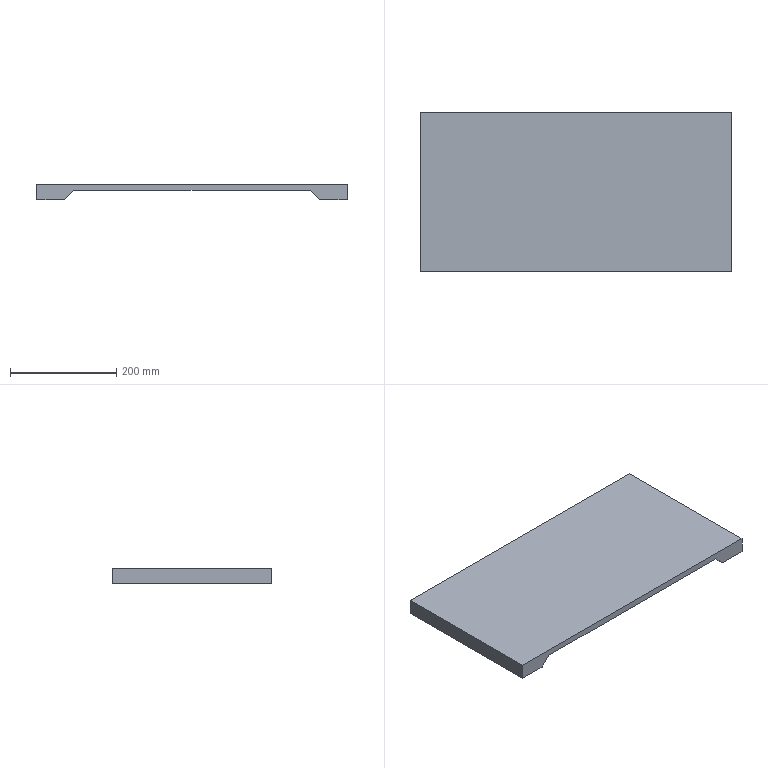Part | STEP file | Platform 2 base plate | 1 solid | 10 faces | box 585 x 300 x 30 mm | volume 2764800 mm3 | plane 10
STEP:
#1=CARTESIAN_POINT('',(240.5,-150.,0.));
#2=VERTEX_POINT('',#1);
#3=CARTESIAN_POINT('',(292.5,-150.,0.));
#4=VERTEX_POINT('',#3);
#5=CARTESIAN_POINT('',(-292.5,-150.,0.));
#6=DIRECTION('',(1.,0.,0.));
#7=VECTOR('',#6,1000.);
#8=LINE('',#5,#7);
#9=EDGE_CURVE('',#2,#4,#8,.T.);
#10=ORIENTED_EDGE('',*,*,#9,.F.);
#11=CARTESIAN_POINT('',(240.5,150.,0.));
#12=VERTEX_POINT('',#11);
#13=CARTESIAN_POINT('',(240.5,150.,0.));
#14=DIRECTION('',(0.,-1.,0.));
#15=VECTOR('',#14,1000.);
#16=LINE('',#13,#15);
#17=EDGE_CURVE('',#12,#2,#16,.T.);
#18=ORIENTED_EDGE('',*,*,#17,.F.);
#19=CARTESIAN_POINT('',(292.5,150.,0.));
#20=VERTEX_POINT('',#19);
#21=CARTESIAN_POINT('',(-292.5,150.,0.));
#22=DIRECTION('',(-1.,0.,0.));
#23=VECTOR('',#22,1000.);
#24=LINE('',#21,#23);
#25=EDGE_CURVE('',#20,#12,#24,.T.);
#26=ORIENTED_EDGE('',*,*,#25,.F.);
#27=CARTESIAN_POINT('',(292.5,150.,0.));
#28=DIRECTION('',(0.,1.,0.));
#29=VECTOR('',#28,1000.);
#30=LINE('',#27,#29);
#31=EDGE_CURVE('',#4,#20,#30,.T.);
#32=ORIENTED_EDGE('',*,*,#31,.F.);
#33=EDGE_LOOP('',(#10,#18,#26,#32));
#34=FACE_OUTER_BOUND('',#33,.T.);
#35=CARTESIAN_POINT('',(0.,0.,0.));
#36=DIRECTION('',(0.,0.,1.));
#37=DIRECTION('',(1.,0.,0.));
#38=AXIS2_PLACEMENT_3D('',#35,#36,#37);
#39=PLANE('',#38);
#40=ADVANCED_FACE('',(#34),#39,.F.);
#41=ORIENTED_EDGE('',*,*,#31,.T.);
#42=CARTESIAN_POINT('',(292.5,150.,30.));
#43=VERTEX_POINT('',#42);
#44=CARTESIAN_POINT('',(292.5,150.,30.));
#45=DIRECTION('',(0.,0.,-1.));
#46=VECTOR('',#45,1000.);
#47=LINE('',#44,#46);
#48=EDGE_CURVE('',#43,#20,#47,.T.);
#49=ORIENTED_EDGE('',*,*,#48,.F.);
#50=CARTESIAN_POINT('',(292.5,-150.,30.));
#51=VERTEX_POINT('',#50);
#52=CARTESIAN_POINT('',(292.5,150.,30.));
#53=DIRECTION('',(0.,1.,0.));
#54=VECTOR('',#53,1000.);
#55=LINE('',#52,#54);
#56=EDGE_CURVE('',#51,#43,#55,.T.);
#57=ORIENTED_EDGE('',*,*,#56,.F.);
#58=CARTESIAN_POINT('',(292.5,-150.,30.));
#59=DIRECTION('',(0.,0.,-1.));
#60=VECTOR('',#59,1000.);
#61=LINE('',#58,#60);
#62=EDGE_CURVE('',#51,#4,#61,.T.);
#63=ORIENTED_EDGE('',*,*,#62,.T.);
#64=EDGE_LOOP('',(#41,#49,#57,#63));
#65=FACE_OUTER_BOUND('',#64,.T.);
#66=CARTESIAN_POINT('',(292.5,150.,30.));
#67=DIRECTION('',(-1.,0.,0.));
#68=DIRECTION('',(0.,0.,1.));
#69=AXIS2_PLACEMENT_3D('',#66,#67,#68);
#70=PLANE('',#69);
#71=ADVANCED_FACE('',(#65),#70,.F.);
#72=ORIENTED_EDGE('',*,*,#25,.T.);
#73=CARTESIAN_POINT('',(222.5,150.,18.));
#74=VERTEX_POINT('',#73);
#75=CARTESIAN_POINT('',(222.5,150.,18.));
#76=DIRECTION('',(-0.7071,0.,0.7071));
#77=VECTOR('',#76,1000.);
#78=LINE('',#75,#77);
#79=EDGE_CURVE('',#12,#74,#78,.T.);
#80=ORIENTED_EDGE('',*,*,#79,.T.);
#81=CARTESIAN_POINT('',(-222.5,150.,18.));
#82=VERTEX_POINT('',#81);
#83=CARTESIAN_POINT('',(-222.5,150.,18.));
#84=DIRECTION('',(-1.,0.,0.));
#85=VECTOR('',#84,1000.);
#86=LINE('',#83,#85);
#87=EDGE_CURVE('',#74,#82,#86,.T.);
#88=ORIENTED_EDGE('',*,*,#87,.T.);
#89=CARTESIAN_POINT('',(-240.5,150.,0.));
#90=VERTEX_POINT('',#89);
#91=CARTESIAN_POINT('',(-222.5,150.,18.));
#92=DIRECTION('',(-0.7071,0.,-0.7071));
#93=VECTOR('',#92,1000.);
#94=LINE('',#91,#93);
#95=EDGE_CURVE('',#82,#90,#94,.T.);
#96=ORIENTED_EDGE('',*,*,#95,.T.);
#97=CARTESIAN_POINT('',(-292.5,150.,0.));
#98=VERTEX_POINT('',#97);
#99=CARTESIAN_POINT('',(-292.5,150.,0.));
#100=DIRECTION('',(-1.,0.,0.));
#101=VECTOR('',#100,1000.);
#102=LINE('',#99,#101);
#103=EDGE_CURVE('',#90,#98,#102,.T.);
#104=ORIENTED_EDGE('',*,*,#103,.T.);
#105=CARTESIAN_POINT('',(-292.5,150.,30.));
#106=VERTEX_POINT('',#105);
#107=CARTESIAN_POINT('',(-292.5,150.,30.));
#108=DIRECTION('',(0.,0.,-1.));
#109=VECTOR('',#108,1000.);
#110=LINE('',#107,#109);
#111=EDGE_CURVE('',#106,#98,#110,.T.);
#112=ORIENTED_EDGE('',*,*,#111,.F.);
#113=CARTESIAN_POINT('',(-292.5,150.,30.));
#114=DIRECTION('',(-1.,0.,0.));
#115=VECTOR('',#114,1000.);
#116=LINE('',#113,#115);
#117=EDGE_CURVE('',#43,#106,#116,.T.);
#118=ORIENTED_EDGE('',*,*,#117,.F.);
#119=ORIENTED_EDGE('',*,*,#48,.T.);
#120=EDGE_LOOP('',(#72,#80,#88,#96,#104,#112,#118,#119));
#121=FACE_OUTER_BOUND('',#120,.T.);
#122=CARTESIAN_POINT('',(-292.5,150.,30.));
#123=DIRECTION('',(0.,-1.,0.));
#124=DIRECTION('',(0.,0.,-1.));
#125=AXIS2_PLACEMENT_3D('',#122,#123,#124);
#126=PLANE('',#125);
#127=ADVANCED_FACE('',(#121),#126,.F.);
#128=CARTESIAN_POINT('',(-292.5,-150.,0.));
#129=VERTEX_POINT('',#128);
#130=CARTESIAN_POINT('',(-292.5,150.,0.));
#131=DIRECTION('',(0.,-1.,0.));
#132=VECTOR('',#131,1000.);
#133=LINE('',#130,#132);
#134=EDGE_CURVE('',#98,#129,#133,.T.);
#135=ORIENTED_EDGE('',*,*,#134,.T.);
#136=CARTESIAN_POINT('',(-292.5,-150.,30.));
#137=VERTEX_POINT('',#136);
#138=CARTESIAN_POINT('',(-292.5,-150.,30.));
#139=DIRECTION('',(0.,0.,-1.));
#140=VECTOR('',#139,1000.);
#141=LINE('',#138,#140);
#142=EDGE_CURVE('',#137,#129,#141,.T.);
#143=ORIENTED_EDGE('',*,*,#142,.F.);
#144=CARTESIAN_POINT('',(-292.5,150.,30.));
#145=DIRECTION('',(0.,-1.,0.));
#146=VECTOR('',#145,1000.);
#147=LINE('',#144,#146);
#148=EDGE_CURVE('',#106,#137,#147,.T.);
#149=ORIENTED_EDGE('',*,*,#148,.F.);
#150=ORIENTED_EDGE('',*,*,#111,.T.);
#151=EDGE_LOOP('',(#135,#143,#149,#150));
#152=FACE_OUTER_BOUND('',#151,.T.);
#153=CARTESIAN_POINT('',(-292.5,150.,30.));
#154=DIRECTION('',(1.,0.,0.));
#155=DIRECTION('',(0.,1.,0.));
#156=AXIS2_PLACEMENT_3D('',#153,#154,#155);
#157=PLANE('',#156);
#158=ADVANCED_FACE('',(#152),#157,.F.);
#159=CARTESIAN_POINT('',(222.5,-150.,18.));
#160=VERTEX_POINT('',#159);
#161=CARTESIAN_POINT('',(-222.5,-150.,18.));
#162=VERTEX_POINT('',#161);
#163=CARTESIAN_POINT('',(-222.5,-150.,18.));
#164=DIRECTION('',(-1.,0.,0.));
#165=VECTOR('',#164,1000.);
#166=LINE('',#163,#165);
#167=EDGE_CURVE('',#160,#162,#166,.T.);
#168=ORIENTED_EDGE('',*,*,#167,.F.);
#169=CARTESIAN_POINT('',(222.5,-150.,18.));
#170=DIRECTION('',(-0.7071,0.,0.7071));
#171=VECTOR('',#170,1000.);
#172=LINE('',#169,#171);
#173=EDGE_CURVE('',#2,#160,#172,.T.);
#174=ORIENTED_EDGE('',*,*,#173,.F.);
#175=ORIENTED_EDGE('',*,*,#9,.T.);
#176=ORIENTED_EDGE('',*,*,#62,.F.);
#177=CARTESIAN_POINT('',(-292.5,-150.,30.));
#178=DIRECTION('',(1.,0.,0.));
#179=VECTOR('',#178,1000.);
#180=LINE('',#177,#179);
#181=EDGE_CURVE('',#137,#51,#180,.T.);
#182=ORIENTED_EDGE('',*,*,#181,.F.);
#183=ORIENTED_EDGE('',*,*,#142,.T.);
#184=CARTESIAN_POINT('',(-240.5,-150.,0.));
#185=VERTEX_POINT('',#184);
#186=CARTESIAN_POINT('',(-292.5,-150.,0.));
#187=DIRECTION('',(1.,0.,0.));
#188=VECTOR('',#187,1000.);
#189=LINE('',#186,#188);
#190=EDGE_CURVE('',#129,#185,#189,.T.);
#191=ORIENTED_EDGE('',*,*,#190,.T.);
#192=CARTESIAN_POINT('',(-222.5,-150.,18.));
#193=DIRECTION('',(-0.7071,0.,-0.7071));
#194=VECTOR('',#193,1000.);
#195=LINE('',#192,#194);
#196=EDGE_CURVE('',#162,#185,#195,.T.);
#197=ORIENTED_EDGE('',*,*,#196,.F.);
#198=EDGE_LOOP('',(#168,#174,#175,#176,#182,#183,#191,#197));
#199=FACE_OUTER_BOUND('',#198,.T.);
#200=CARTESIAN_POINT('',(-292.5,-150.,30.));
#201=DIRECTION('',(0.,1.,0.));
#202=DIRECTION('',(0.,0.,1.));
#203=AXIS2_PLACEMENT_3D('',#200,#201,#202);
#204=PLANE('',#203);
#205=ADVANCED_FACE('',(#199),#204,.F.);
#206=ORIENTED_EDGE('',*,*,#56,.T.);
#207=ORIENTED_EDGE('',*,*,#117,.T.);
#208=ORIENTED_EDGE('',*,*,#148,.T.);
#209=ORIENTED_EDGE('',*,*,#181,.T.);
#210=EDGE_LOOP('',(#206,#207,#208,#209));
#211=FACE_OUTER_BOUND('',#210,.T.);
#212=CARTESIAN_POINT('',(0.,0.,30.));
#213=DIRECTION('',(0.,0.,1.));
#214=DIRECTION('',(1.,0.,0.));
#215=AXIS2_PLACEMENT_3D('',#212,#213,#214);
#216=PLANE('',#215);
#217=ADVANCED_FACE('',(#211),#216,.T.);
#218=ORIENTED_EDGE('',*,*,#103,.F.);
#219=CARTESIAN_POINT('',(-240.5,150.,0.));
#220=DIRECTION('',(0.,-1.,0.));
#221=VECTOR('',#220,1000.);
#222=LINE('',#219,#221);
#223=EDGE_CURVE('',#90,#185,#222,.T.);
#224=ORIENTED_EDGE('',*,*,#223,.T.);
#225=ORIENTED_EDGE('',*,*,#190,.F.);
#226=ORIENTED_EDGE('',*,*,#134,.F.);
#227=EDGE_LOOP('',(#218,#224,#225,#226));
#228=FACE_OUTER_BOUND('',#227,.T.);
#229=CARTESIAN_POINT('',(0.,0.,0.));
#230=DIRECTION('',(0.,0.,1.));
#231=DIRECTION('',(1.,0.,0.));
#232=AXIS2_PLACEMENT_3D('',#229,#230,#231);
#233=PLANE('',#232);
#234=ADVANCED_FACE('',(#228),#233,.F.);
#235=ORIENTED_EDGE('',*,*,#173,.T.);
#236=CARTESIAN_POINT('',(222.5,150.,18.));
#237=DIRECTION('',(0.,-1.,0.));
#238=VECTOR('',#237,1000.);
#239=LINE('',#236,#238);
#240=EDGE_CURVE('',#74,#160,#239,.T.);
#241=ORIENTED_EDGE('',*,*,#240,.F.);
#242=ORIENTED_EDGE('',*,*,#79,.F.);
#243=ORIENTED_EDGE('',*,*,#17,.T.);
#244=EDGE_LOOP('',(#235,#241,#242,#243));
#245=FACE_OUTER_BOUND('',#244,.T.);
#246=CARTESIAN_POINT('',(222.5,150.,18.));
#247=DIRECTION('',(0.7071,0.,0.7071));
#248=DIRECTION('',(0.7071,0.,-0.7071));
#249=AXIS2_PLACEMENT_3D('',#246,#247,#248);
#250=PLANE('',#249);
#251=ADVANCED_FACE('',(#245),#250,.F.);
#252=ORIENTED_EDGE('',*,*,#196,.T.);
#253=ORIENTED_EDGE('',*,*,#223,.F.);
#254=ORIENTED_EDGE('',*,*,#95,.F.);
#255=CARTESIAN_POINT('',(-222.5,150.,18.));
#256=DIRECTION('',(0.,-1.,0.));
#257=VECTOR('',#256,1000.);
#258=LINE('',#255,#257);
#259=EDGE_CURVE('',#82,#162,#258,.T.);
#260=ORIENTED_EDGE('',*,*,#259,.T.);
#261=EDGE_LOOP('',(#252,#253,#254,#260));
#262=FACE_OUTER_BOUND('',#261,.T.);
#263=CARTESIAN_POINT('',(-222.5,150.,18.));
#264=DIRECTION('',(-0.7071,0.,0.7071));
#265=DIRECTION('',(0.7071,0.,0.7071));
#266=AXIS2_PLACEMENT_3D('',#263,#264,#265);
#267=PLANE('',#266);
#268=ADVANCED_FACE('',(#262),#267,.F.);
#269=ORIENTED_EDGE('',*,*,#167,.T.);
#270=ORIENTED_EDGE('',*,*,#259,.F.);
#271=ORIENTED_EDGE('',*,*,#87,.F.);
#272=ORIENTED_EDGE('',*,*,#240,.T.);
#273=EDGE_LOOP('',(#269,#270,#271,#272));
#274=FACE_OUTER_BOUND('',#273,.T.);
#275=CARTESIAN_POINT('',(-222.5,150.,18.));
#276=DIRECTION('',(0.,0.,1.));
#277=DIRECTION('',(1.,0.,0.));
#278=AXIS2_PLACEMENT_3D('',#275,#276,#277);
#279=PLANE('',#278);
#280=ADVANCED_FACE('',(#274),#279,.F.);
#281=CLOSED_SHELL('',(#40,#71,#127,#158,#205,#217,#234,#251,#268,#280));
#282=MANIFOLD_SOLID_BREP('',#281);
#283=CARTESIAN_POINT('',(0.,0.,0.));
#284=DIRECTION('',(0.,0.,1.));
#285=DIRECTION('',(1.,0.,0.));
#286=AXIS2_PLACEMENT_3D('',#283,#284,#285);
#287=(LENGTH_UNIT()NAMED_UNIT(*)SI_UNIT(.MILLI.,.METRE.));
#288=UNCERTAINTY_MEASURE_WITH_UNIT(LENGTH_MEASURE(0.00001),#287,'','');
#289=(NAMED_UNIT(*)PLANE_ANGLE_UNIT()SI_UNIT($,.RADIAN.));
#290=(NAMED_UNIT(*)SI_UNIT($,.STERADIAN.)SOLID_ANGLE_UNIT());
#291=(GEOMETRIC_REPRESENTATION_CONTEXT(3)GLOBAL_UNCERTAINTY_ASSIGNED_CONTEXT((#288))GLOBAL_UNIT_ASSIGNED_CONTEXT((#287,#289,#290))REPRESENTATION_CONTEXT('',''));
#292=ADVANCED_BREP_SHAPE_REPRESENTATION('',(#282,#286),#291);